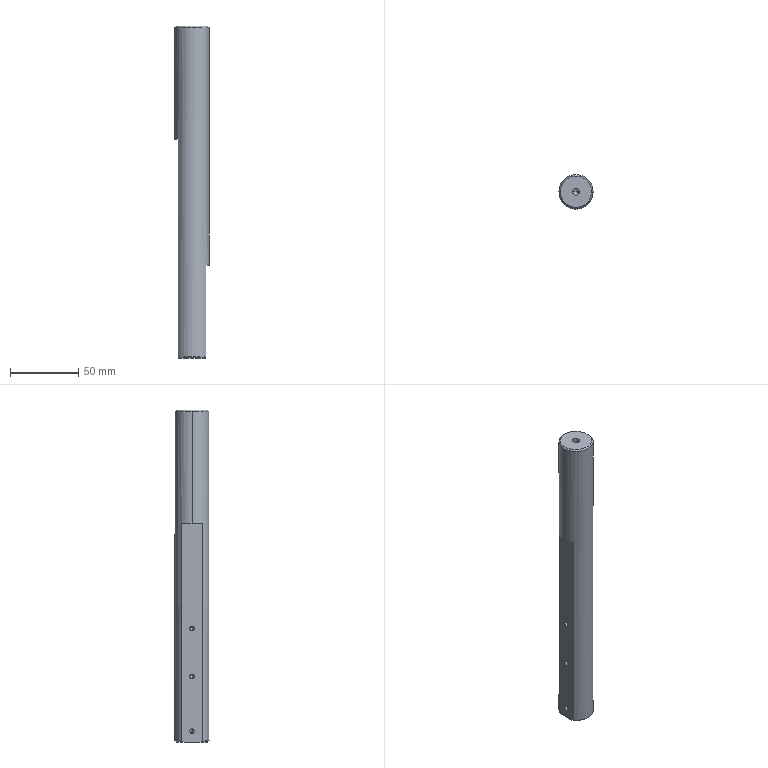Part | SolidWorks | features HoleWzd 3, ICE 3, Chamfer 1, Extrusion 1 | 1 solid | 39 faces | box 25 x 25 x 243 mm | volume 111932 mm3 | cone 16 | cylinder 16 | plane 7 | commonest cylinder face diameters 3.3 x6 5 x6 6 x2 25 x2
STEP:
#1=CARTESIAN_POINT('',(11.5,0.,243.));
#2=VERTEX_POINT('',#1);
#3=CARTESIAN_POINT('',(-11.5,0.,243.));
#4=VERTEX_POINT('',#3);
#5=CARTESIAN_POINT('',(0.,0.,243.));
#6=DIRECTION('',(0.,0.,1.));
#7=DIRECTION('',(1.,0.,0.));
#8=AXIS2_PLACEMENT_3D('',#5,#6,#7);
#9=CIRCLE('',#8,11.5);
#10=EDGE_CURVE('',#2,#4,#9,.T.);
#11=ORIENTED_EDGE('',*,*,#10,.F.);
#12=CARTESIAN_POINT('',(12.5,0.,242.));
#13=VERTEX_POINT('',#12);
#14=CARTESIAN_POINT('',(11.5,0.,243.));
#15=DIRECTION('',(0.7071,0.,-0.7071));
#16=VECTOR('',#15,1000.);
#17=LINE('',#14,#16);
#18=EDGE_CURVE('',#2,#13,#17,.T.);
#19=ORIENTED_EDGE('',*,*,#18,.T.);
#20=CARTESIAN_POINT('',(-12.5,0.,242.));
#21=VERTEX_POINT('',#20);
#22=CARTESIAN_POINT('',(0.,0.,242.));
#23=DIRECTION('',(0.,0.,-1.));
#24=DIRECTION('',(1.,0.,0.));
#25=AXIS2_PLACEMENT_3D('',#22,#23,#24);
#26=CIRCLE('',#25,12.5);
#27=EDGE_CURVE('',#21,#13,#26,.T.);
#28=ORIENTED_EDGE('',*,*,#27,.F.);
#29=CARTESIAN_POINT('',(-11.5,0.,243.));
#30=DIRECTION('',(-0.7071,0.,-0.7071));
#31=VECTOR('',#30,1000.);
#32=LINE('',#29,#31);
#33=EDGE_CURVE('',#4,#21,#32,.T.);
#34=ORIENTED_EDGE('',*,*,#33,.F.);
#35=EDGE_LOOP('',(#11,#19,#28,#34));
#36=FACE_OUTER_BOUND('',#35,.T.);
#37=CARTESIAN_POINT('',(0.,0.,243.));
#38=DIRECTION('',(0.,0.,-1.));
#39=DIRECTION('',(-1.,0.,0.));
#40=AXIS2_PLACEMENT_3D('',#37,#38,#39);
#41=CONICAL_SURFACE('',#40,11.5,0.7854);
#42=ADVANCED_FACE('',(#36),#41,.T.);
#43=CARTESIAN_POINT('',(0.,0.,36.));
#44=VERTEX_POINT('',#43);
#45=CARTESIAN_POINT('',(0.,0.,30.));
#46=VERTEX_POINT('',#45);
#47=CARTESIAN_POINT('',(0.,0.,33.));
#48=DIRECTION('',(1.,0.,0.));
#49=DIRECTION('',(0.,0.,-1.));
#50=AXIS2_PLACEMENT_3D('',#47,#48,#49);
#51=CIRCLE('',#50,3.);
#52=EDGE_CURVE('',#44,#46,#51,.T.);
#53=ORIENTED_EDGE('',*,*,#52,.F.);
#54=CARTESIAN_POINT('',(10.,0.,36.));
#55=VERTEX_POINT('',#54);
#56=CARTESIAN_POINT('',(0.,0.,36.));
#57=DIRECTION('',(1.,0.,0.));
#58=VECTOR('',#57,1000.);
#59=LINE('',#56,#58);
#60=EDGE_CURVE('',#44,#55,#59,.T.);
#61=ORIENTED_EDGE('',*,*,#60,.T.);
#62=CARTESIAN_POINT('',(10.,0.,30.));
#63=VERTEX_POINT('',#62);
#64=CARTESIAN_POINT('',(10.,0.,33.));
#65=DIRECTION('',(1.,0.,0.));
#66=DIRECTION('',(0.,0.,-1.));
#67=AXIS2_PLACEMENT_3D('',#64,#65,#66);
#68=CIRCLE('',#67,3.);
#69=EDGE_CURVE('',#55,#63,#68,.T.);
#70=ORIENTED_EDGE('',*,*,#69,.T.);
#71=CARTESIAN_POINT('',(0.,0.,30.));
#72=DIRECTION('',(1.,0.,0.));
#73=VECTOR('',#72,1000.);
#74=LINE('',#71,#73);
#75=EDGE_CURVE('',#46,#63,#74,.T.);
#76=ORIENTED_EDGE('',*,*,#75,.F.);
#77=EDGE_LOOP('',(#53,#61,#70,#76));
#78=FACE_OUTER_BOUND('',#77,.T.);
#79=CARTESIAN_POINT('',(0.,0.,33.));
#80=DIRECTION('',(1.,0.,0.));
#81=DIRECTION('',(0.,0.,-1.));
#82=AXIS2_PLACEMENT_3D('',#79,#80,#81);
#83=CYLINDRICAL_SURFACE('',#82,3.);
#84=ADVANCED_FACE('',(#78),#83,.F.);
#85=CARTESIAN_POINT('',(0.1,0.,6.35));
#86=VERTEX_POINT('',#85);
#87=CARTESIAN_POINT('',(0.1,0.,9.65));
#88=VERTEX_POINT('',#87);
#89=CARTESIAN_POINT('',(0.1,0.,8.));
#90=DIRECTION('',(-1.,0.,0.));
#91=DIRECTION('',(0.,0.,1.));
#92=AXIS2_PLACEMENT_3D('',#89,#90,#91);
#93=CIRCLE('',#92,1.65);
#94=EDGE_CURVE('',#86,#88,#93,.T.);
#95=ORIENTED_EDGE('',*,*,#94,.F.);
#96=CARTESIAN_POINT('',(-10.,0.,6.35));
#97=VERTEX_POINT('',#96);
#98=CARTESIAN_POINT('',(-10.,0.,6.35));
#99=DIRECTION('',(-1.,0.,0.));
#100=VECTOR('',#99,1000.);
#101=LINE('',#98,#100);
#102=EDGE_CURVE('',#86,#97,#101,.T.);
#103=ORIENTED_EDGE('',*,*,#102,.T.);
#104=CARTESIAN_POINT('',(-10.,0.,9.65));
#105=VERTEX_POINT('',#104);
#106=CARTESIAN_POINT('',(-10.,0.,8.));
#107=DIRECTION('',(-1.,0.,0.));
#108=DIRECTION('',(0.,0.,1.));
#109=AXIS2_PLACEMENT_3D('',#106,#107,#108);
#110=CIRCLE('',#109,1.65);
#111=EDGE_CURVE('',#97,#105,#110,.T.);
#112=ORIENTED_EDGE('',*,*,#111,.T.);
#113=CARTESIAN_POINT('',(-10.,0.,9.65));
#114=DIRECTION('',(-1.,0.,0.));
#115=VECTOR('',#114,1000.);
#116=LINE('',#113,#115);
#117=EDGE_CURVE('',#88,#105,#116,.T.);
#118=ORIENTED_EDGE('',*,*,#117,.F.);
#119=EDGE_LOOP('',(#95,#103,#112,#118));
#120=FACE_OUTER_BOUND('',#119,.T.);
#121=CARTESIAN_POINT('',(-10.,0.,8.));
#122=DIRECTION('',(-1.,0.,0.));
#123=DIRECTION('',(0.,0.,1.));
#124=AXIS2_PLACEMENT_3D('',#121,#122,#123);
#125=CYLINDRICAL_SURFACE('',#124,1.65);
#126=ADVANCED_FACE('',(#120),#125,.F.);
#127=CARTESIAN_POINT('',(1.091,0.,8.));
#128=VERTEX_POINT('',#127);
#129=CARTESIAN_POINT('',(0.1,0.,9.65));
#130=DIRECTION('',(-0.515,0.,0.8572));
#131=VECTOR('',#130,1000.);
#132=LINE('',#129,#131);
#133=EDGE_CURVE('',#128,#88,#132,.T.);
#134=ORIENTED_EDGE('',*,*,#133,.F.);
#135=CARTESIAN_POINT('',(0.1,0.,6.35));
#136=DIRECTION('',(-0.515,0.,-0.8572));
#137=VECTOR('',#136,1000.);
#138=LINE('',#135,#137);
#139=EDGE_CURVE('',#128,#86,#138,.T.);
#140=ORIENTED_EDGE('',*,*,#139,.T.);
#141=ORIENTED_EDGE('',*,*,#94,.T.);
#142=EDGE_LOOP('',(#134,#140,#141));
#143=FACE_OUTER_BOUND('',#142,.T.);
#144=CARTESIAN_POINT('',(0.1,0.,8.));
#145=DIRECTION('',(-1.,0.,0.));
#146=DIRECTION('',(0.,0.,1.));
#147=AXIS2_PLACEMENT_3D('',#144,#145,#146);
#148=CONICAL_SURFACE('',#147,1.65,1.03);
#149=ADVANCED_FACE('',(#143),#148,.F.);
#150=CARTESIAN_POINT('',(0.1,0.,81.35));
#151=VERTEX_POINT('',#150);
#152=CARTESIAN_POINT('',(0.1,0.,84.65));
#153=VERTEX_POINT('',#152);
#154=CARTESIAN_POINT('',(0.1,0.,83.));
#155=DIRECTION('',(-1.,0.,0.));
#156=DIRECTION('',(0.,0.,1.));
#157=AXIS2_PLACEMENT_3D('',#154,#155,#156);
#158=CIRCLE('',#157,1.65);
#159=EDGE_CURVE('',#151,#153,#158,.T.);
#160=ORIENTED_EDGE('',*,*,#159,.F.);
#161=CARTESIAN_POINT('',(-10.,0.,81.35));
#162=VERTEX_POINT('',#161);
#163=CARTESIAN_POINT('',(-10.,0.,81.35));
#164=DIRECTION('',(-1.,0.,0.));
#165=VECTOR('',#164,1000.);
#166=LINE('',#163,#165);
#167=EDGE_CURVE('',#151,#162,#166,.T.);
#168=ORIENTED_EDGE('',*,*,#167,.T.);
#169=CARTESIAN_POINT('',(-10.,0.,84.65));
#170=VERTEX_POINT('',#169);
#171=CARTESIAN_POINT('',(-10.,0.,83.));
#172=DIRECTION('',(-1.,0.,0.));
#173=DIRECTION('',(0.,0.,1.));
#174=AXIS2_PLACEMENT_3D('',#171,#172,#173);
#175=CIRCLE('',#174,1.65);
#176=EDGE_CURVE('',#162,#170,#175,.T.);
#177=ORIENTED_EDGE('',*,*,#176,.T.);
#178=CARTESIAN_POINT('',(-10.,0.,84.65));
#179=DIRECTION('',(-1.,0.,0.));
#180=VECTOR('',#179,1000.);
#181=LINE('',#178,#180);
#182=EDGE_CURVE('',#153,#170,#181,.T.);
#183=ORIENTED_EDGE('',*,*,#182,.F.);
#184=EDGE_LOOP('',(#160,#168,#177,#183));
#185=FACE_OUTER_BOUND('',#184,.T.);
#186=CARTESIAN_POINT('',(-10.,0.,83.));
#187=DIRECTION('',(-1.,0.,0.));
#188=DIRECTION('',(0.,0.,1.));
#189=AXIS2_PLACEMENT_3D('',#186,#187,#188);
#190=CYLINDRICAL_SURFACE('',#189,1.65);
#191=ADVANCED_FACE('',(#185),#190,.F.);
#192=CARTESIAN_POINT('',(1.091,0.,83.));
#193=VERTEX_POINT('',#192);
#194=CARTESIAN_POINT('',(0.1,0.,84.65));
#195=DIRECTION('',(-0.515,0.,0.8572));
#196=VECTOR('',#195,1000.);
#197=LINE('',#194,#196);
#198=EDGE_CURVE('',#193,#153,#197,.T.);
#199=ORIENTED_EDGE('',*,*,#198,.F.);
#200=CARTESIAN_POINT('',(0.1,0.,81.35));
#201=DIRECTION('',(-0.515,0.,-0.8572));
#202=VECTOR('',#201,1000.);
#203=LINE('',#200,#202);
#204=EDGE_CURVE('',#193,#151,#203,.T.);
#205=ORIENTED_EDGE('',*,*,#204,.T.);
#206=ORIENTED_EDGE('',*,*,#159,.T.);
#207=EDGE_LOOP('',(#199,#205,#206));
#208=FACE_OUTER_BOUND('',#207,.T.);
#209=CARTESIAN_POINT('',(0.1,0.,83.));
#210=DIRECTION('',(-1.,0.,0.));
#211=DIRECTION('',(0.,0.,1.));
#212=AXIS2_PLACEMENT_3D('',#209,#210,#211);
#213=CONICAL_SURFACE('',#212,1.65,1.03);
#214=ADVANCED_FACE('',(#208),#213,.F.);
#215=CARTESIAN_POINT('',(0.1,0.,46.35));
#216=VERTEX_POINT('',#215);
#217=CARTESIAN_POINT('',(0.1,0.,49.65));
#218=VERTEX_POINT('',#217);
#219=CARTESIAN_POINT('',(0.1,0.,48.));
#220=DIRECTION('',(-1.,0.,0.));
#221=DIRECTION('',(0.,0.,1.));
#222=AXIS2_PLACEMENT_3D('',#219,#220,#221);
#223=CIRCLE('',#222,1.65);
#224=EDGE_CURVE('',#216,#218,#223,.T.);
#225=ORIENTED_EDGE('',*,*,#224,.F.);
#226=CARTESIAN_POINT('',(-10.,0.,46.35));
#227=VERTEX_POINT('',#226);
#228=CARTESIAN_POINT('',(-10.,0.,46.35));
#229=DIRECTION('',(-1.,0.,0.));
#230=VECTOR('',#229,1000.);
#231=LINE('',#228,#230);
#232=EDGE_CURVE('',#216,#227,#231,.T.);
#233=ORIENTED_EDGE('',*,*,#232,.T.);
#234=CARTESIAN_POINT('',(-10.,0.,49.65));
#235=VERTEX_POINT('',#234);
#236=CARTESIAN_POINT('',(-10.,0.,48.));
#237=DIRECTION('',(-1.,0.,0.));
#238=DIRECTION('',(0.,0.,1.));
#239=AXIS2_PLACEMENT_3D('',#236,#237,#238);
#240=CIRCLE('',#239,1.65);
#241=EDGE_CURVE('',#227,#235,#240,.T.);
#242=ORIENTED_EDGE('',*,*,#241,.T.);
#243=CARTESIAN_POINT('',(-10.,0.,49.65));
#244=DIRECTION('',(-1.,0.,0.));
#245=VECTOR('',#244,1000.);
#246=LINE('',#243,#245);
#247=EDGE_CURVE('',#218,#235,#246,.T.);
#248=ORIENTED_EDGE('',*,*,#247,.F.);
#249=EDGE_LOOP('',(#225,#233,#242,#248));
#250=FACE_OUTER_BOUND('',#249,.T.);
#251=CARTESIAN_POINT('',(-10.,0.,48.));
#252=DIRECTION('',(-1.,0.,0.));
#253=DIRECTION('',(0.,0.,1.));
#254=AXIS2_PLACEMENT_3D('',#251,#252,#253);
#255=CYLINDRICAL_SURFACE('',#254,1.65);
#256=ADVANCED_FACE('',(#250),#255,.F.);
#257=CARTESIAN_POINT('',(1.091,0.,48.));
#258=VERTEX_POINT('',#257);
#259=CARTESIAN_POINT('',(0.1,0.,49.65));
#260=DIRECTION('',(-0.515,0.,0.8572));
#261=VECTOR('',#260,1000.);
#262=LINE('',#259,#261);
#263=EDGE_CURVE('',#258,#218,#262,.T.);
#264=ORIENTED_EDGE('',*,*,#263,.F.);
#265=CARTESIAN_POINT('',(0.1,0.,46.35));
#266=DIRECTION('',(-0.515,0.,-0.8572));
#267=VECTOR('',#266,1000.);
#268=LINE('',#265,#267);
#269=EDGE_CURVE('',#258,#216,#268,.T.);
#270=ORIENTED_EDGE('',*,*,#269,.T.);
#271=ORIENTED_EDGE('',*,*,#224,.T.);
#272=EDGE_LOOP('',(#264,#270,#271));
#273=FACE_OUTER_BOUND('',#272,.T.);
#274=CARTESIAN_POINT('',(0.1,0.,48.));
#275=DIRECTION('',(-1.,0.,0.));
#276=DIRECTION('',(0.,0.,1.));
#277=AXIS2_PLACEMENT_3D('',#274,#275,#276);
#278=CONICAL_SURFACE('',#277,1.65,1.03);
#279=ADVANCED_FACE('',(#273),#278,.F.);
#280=CARTESIAN_POINT('',(-5.,0.,15.5));
#281=VERTEX_POINT('',#280);
#282=CARTESIAN_POINT('',(-5.,0.,10.5));
#283=VERTEX_POINT('',#282);
#284=CARTESIAN_POINT('',(-5.,0.,13.));
#285=DIRECTION('',(1.,0.,0.));
#286=DIRECTION('',(0.,0.,-1.));
#287=AXIS2_PLACEMENT_3D('',#284,#285,#286);
#288=CIRCLE('',#287,2.5);
#289=EDGE_CURVE('',#281,#283,#288,.T.);
#290=ORIENTED_EDGE('',*,*,#289,.F.);
#291=CARTESIAN_POINT('',(10.,0.,15.5));
#292=VERTEX_POINT('',#291);
#293=CARTESIAN_POINT('',(10.,0.,15.5));
#294=DIRECTION('',(1.,0.,0.));
#295=VECTOR('',#294,1000.);
#296=LINE('',#293,#295);
#297=EDGE_CURVE('',#281,#292,#296,.T.);
#298=ORIENTED_EDGE('',*,*,#297,.T.);
#299=CARTESIAN_POINT('',(10.,0.,10.5));
#300=VERTEX_POINT('',#299);
#301=CARTESIAN_POINT('',(10.,0.,13.));
#302=DIRECTION('',(1.,0.,0.));
#303=DIRECTION('',(0.,0.,-1.));
#304=AXIS2_PLACEMENT_3D('',#301,#302,#303);
#305=CIRCLE('',#304,2.5);
#306=EDGE_CURVE('',#292,#300,#305,.T.);
#307=ORIENTED_EDGE('',*,*,#306,.T.);
#308=CARTESIAN_POINT('',(10.,0.,10.5));
#309=DIRECTION('',(1.,0.,0.));
#310=VECTOR('',#309,1000.);
#311=LINE('',#308,#310);
#312=EDGE_CURVE('',#283,#300,#311,.T.);
#313=ORIENTED_EDGE('',*,*,#312,.F.);
#314=EDGE_LOOP('',(#290,#298,#307,#313));
#315=FACE_OUTER_BOUND('',#314,.T.);
#316=CARTESIAN_POINT('',(10.,0.,13.));
#317=DIRECTION('',(1.,0.,0.));
#318=DIRECTION('',(0.,0.,-1.));
#319=AXIS2_PLACEMENT_3D('',#316,#317,#318);
#320=CYLINDRICAL_SURFACE('',#319,2.5);
#321=ADVANCED_FACE('',(#315),#320,.F.);
#322=CARTESIAN_POINT('',(-6.502,0.,13.));
#323=VERTEX_POINT('',#322);
#324=CARTESIAN_POINT('',(-5.,0.,10.5));
#325=DIRECTION('',(0.515,0.,-0.8572));
#326=VECTOR('',#325,1000.);
#327=LINE('',#324,#326);
#328=EDGE_CURVE('',#323,#283,#327,.T.);
#329=ORIENTED_EDGE('',*,*,#328,.F.);
#330=CARTESIAN_POINT('',(-5.,0.,15.5));
#331=DIRECTION('',(0.515,0.,0.8572));
#332=VECTOR('',#331,1000.);
#333=LINE('',#330,#332);
#334=EDGE_CURVE('',#323,#281,#333,.T.);
#335=ORIENTED_EDGE('',*,*,#334,.T.);
#336=ORIENTED_EDGE('',*,*,#289,.T.);
#337=EDGE_LOOP('',(#329,#335,#336));
#338=FACE_OUTER_BOUND('',#337,.T.);
#339=CARTESIAN_POINT('',(-5.,0.,13.));
#340=DIRECTION('',(1.,0.,0.));
#341=DIRECTION('',(0.,0.,-1.));
#342=AXIS2_PLACEMENT_3D('',#339,#340,#341);
#343=CONICAL_SURFACE('',#342,2.5,1.03);
#344=ADVANCED_FACE('',(#338),#343,.F.);
#345=CARTESIAN_POINT('',(-5.,0.,55.5));
#346=VERTEX_POINT('',#345);
#347=CARTESIAN_POINT('',(-5.,0.,50.5));
#348=VERTEX_POINT('',#347);
#349=CARTESIAN_POINT('',(-5.,0.,53.));
#350=DIRECTION('',(1.,0.,0.));
#351=DIRECTION('',(0.,0.,-1.));
#352=AXIS2_PLACEMENT_3D('',#349,#350,#351);
#353=CIRCLE('',#352,2.5);
#354=EDGE_CURVE('',#346,#348,#353,.T.);
#355=ORIENTED_EDGE('',*,*,#354,.F.);
#356=CARTESIAN_POINT('',(10.,0.,55.5));
#357=VERTEX_POINT('',#356);
#358=CARTESIAN_POINT('',(10.,0.,55.5));
#359=DIRECTION('',(1.,0.,0.));
#360=VECTOR('',#359,1000.);
#361=LINE('',#358,#360);
#362=EDGE_CURVE('',#346,#357,#361,.T.);
#363=ORIENTED_EDGE('',*,*,#362,.T.);
#364=CARTESIAN_POINT('',(10.,0.,50.5));
#365=VERTEX_POINT('',#364);
#366=CARTESIAN_POINT('',(10.,0.,53.));
#367=DIRECTION('',(1.,0.,0.));
#368=DIRECTION('',(0.,0.,-1.));
#369=AXIS2_PLACEMENT_3D('',#366,#367,#368);
#370=CIRCLE('',#369,2.5);
#371=EDGE_CURVE('',#357,#365,#370,.T.);
#372=ORIENTED_EDGE('',*,*,#371,.T.);
#373=CARTESIAN_POINT('',(10.,0.,50.5));
#374=DIRECTION('',(1.,0.,0.));
#375=VECTOR('',#374,1000.);
#376=LINE('',#373,#375);
#377=EDGE_CURVE('',#348,#365,#376,.T.);
#378=ORIENTED_EDGE('',*,*,#377,.F.);
#379=EDGE_LOOP('',(#355,#363,#372,#378));
#380=FACE_OUTER_BOUND('',#379,.T.);
#381=CARTESIAN_POINT('',(10.,0.,53.));
#382=DIRECTION('',(1.,0.,0.));
#383=DIRECTION('',(0.,0.,-1.));
#384=AXIS2_PLACEMENT_3D('',#381,#382,#383);
#385=CYLINDRICAL_SURFACE('',#384,2.5);
#386=ADVANCED_FACE('',(#380),#385,.F.);
#387=CARTESIAN_POINT('',(-6.502,0.,53.));
#388=VERTEX_POINT('',#387);
#389=CARTESIAN_POINT('',(-5.,0.,50.5));
#390=DIRECTION('',(0.515,0.,-0.8572));
#391=VECTOR('',#390,1000.);
#392=LINE('',#389,#391);
#393=EDGE_CURVE('',#388,#348,#392,.T.);
#394=ORIENTED_EDGE('',*,*,#393,.F.);
#395=CARTESIAN_POINT('',(-5.,0.,55.5));
#396=DIRECTION('',(0.515,0.,0.8572));
#397=VECTOR('',#396,1000.);
#398=LINE('',#395,#397);
#399=EDGE_CURVE('',#388,#346,#398,.T.);
#400=ORIENTED_EDGE('',*,*,#399,.T.);
#401=ORIENTED_EDGE('',*,*,#354,.T.);
#402=EDGE_LOOP('',(#394,#400,#401));
#403=FACE_OUTER_BOUND('',#402,.T.);
#404=CARTESIAN_POINT('',(-5.,0.,53.));
#405=DIRECTION('',(1.,0.,0.));
#406=DIRECTION('',(0.,0.,-1.));
#407=AXIS2_PLACEMENT_3D('',#404,#405,#406);
#408=CONICAL_SURFACE('',#407,2.5,1.03);
#409=ADVANCED_FACE('',(#403),#408,.F.);
#410=CARTESIAN_POINT('',(-2.5,0.,228.));
#411=VERTEX_POINT('',#410);
#412=CARTESIAN_POINT('',(2.5,0.,228.));
#413=VERTEX_POINT('',#412);
#414=CARTESIAN_POINT('',(0.,0.,228.));
#415=DIRECTION('',(0.,0.,1.));
#416=DIRECTION('',(1.,0.,0.));
#417=AXIS2_PLACEMENT_3D('',#414,#415,#416);
#418=CIRCLE('',#417,2.5);
#419=EDGE_CURVE('',#411,#413,#418,.T.);
#420=ORIENTED_EDGE('',*,*,#419,.F.);
#421=CARTESIAN_POINT('',(-2.5,0.,243.));
#422=VERTEX_POINT('',#421);
#423=CARTESIAN_POINT('',(-2.5,0.,243.));
#424=DIRECTION('',(0.,0.,1.));
#425=VECTOR('',#424,1000.);
#426=LINE('',#423,#425);
#427=EDGE_CURVE('',#411,#422,#426,.T.);
#428=ORIENTED_EDGE('',*,*,#427,.T.);
#429=CARTESIAN_POINT('',(2.5,0.,243.));
#430=VERTEX_POINT('',#429);
#431=CARTESIAN_POINT('',(0.,0.,243.));
#432=DIRECTION('',(0.,0.,1.));
#433=DIRECTION('',(1.,0.,0.));
#434=AXIS2_PLACEMENT_3D('',#431,#432,#433);
#435=CIRCLE('',#434,2.5);
#436=EDGE_CURVE('',#422,#430,#435,.T.);
#437=ORIENTED_EDGE('',*,*,#436,.T.);
#438=CARTESIAN_POINT('',(2.5,0.,243.));
#439=DIRECTION('',(0.,0.,1.));
#440=VECTOR('',#439,1000.);
#441=LINE('',#438,#440);
#442=EDGE_CURVE('',#413,#430,#441,.T.);
#443=ORIENTED_EDGE('',*,*,#442,.F.);
#444=EDGE_LOOP('',(#420,#428,#437,#443));
#445=FACE_OUTER_BOUND('',#444,.T.);
#446=CARTESIAN_POINT('',(0.,0.,243.));
#447=DIRECTION('',(0.,0.,1.));
#448=DIRECTION('',(1.,0.,0.));
#449=AXIS2_PLACEMENT_3D('',#446,#447,#448);
#450=CYLINDRICAL_SURFACE('',#449,2.5);
#451=ADVANCED_FACE('',(#445),#450,.F.);
#452=CARTESIAN_POINT('',(0.,0.,226.498));
#453=VERTEX_POINT('',#452);
#454=CARTESIAN_POINT('',(2.5,0.,228.));
#455=DIRECTION('',(0.8572,0.,0.515));
#456=VECTOR('',#455,1000.);
#457=LINE('',#454,#456);
#458=EDGE_CURVE('',#453,#413,#457,.T.);
#459=ORIENTED_EDGE('',*,*,#458,.F.);
#460=CARTESIAN_POINT('',(-2.5,0.,228.));
#461=DIRECTION('',(-0.8572,0.,0.515));
#462=VECTOR('',#461,1000.);
#463=LINE('',#460,#462);
#464=EDGE_CURVE('',#453,#411,#463,.T.);
#465=ORIENTED_EDGE('',*,*,#464,.T.);
#466=ORIENTED_EDGE('',*,*,#419,.T.);
#467=EDGE_LOOP('',(#459,#465,#466));
#468=FACE_OUTER_BOUND('',#467,.T.);
#469=CARTESIAN_POINT('',(0.,0.,228.));
#470=DIRECTION('',(0.,0.,1.));
#471=DIRECTION('',(1.,0.,0.));
#472=AXIS2_PLACEMENT_3D('',#469,#470,#471);
#473=CONICAL_SURFACE('',#472,2.5,1.03);
#474=ADVANCED_FACE('',(#468),#473,.F.);
#475=ORIENTED_EDGE('',*,*,#27,.T.);
#476=CARTESIAN_POINT('',(12.5,0.,68.));
#477=VERTEX_POINT('',#476);
#478=CARTESIAN_POINT('',(12.5,0.,243.));
#479=DIRECTION('',(0.,0.,-1.));
#480=VECTOR('',#479,1000.);
#481=LINE('',#478,#480);
#482=EDGE_CURVE('',#13,#477,#481,.T.);
#483=ORIENTED_EDGE('',*,*,#482,.T.);
#484=CARTESIAN_POINT('',(10.,7.5,68.));
#485=VERTEX_POINT('',#484);
#486=CARTESIAN_POINT('',(0.,0.,68.));
#487=DIRECTION('',(0.,0.,1.));
#488=DIRECTION('',(1.,0.,0.));
#489=AXIS2_PLACEMENT_3D('',#486,#487,#488);
#490=CIRCLE('',#489,12.5);
#491=EDGE_CURVE('',#477,#485,#490,.T.);
#492=ORIENTED_EDGE('',*,*,#491,.T.);
#493=CARTESIAN_POINT('',(10.,7.5,1.));
#494=VERTEX_POINT('',#493);
#495=CARTESIAN_POINT('',(10.,7.5,68.));
#496=DIRECTION('',(0.,0.,-1.));
#497=VECTOR('',#496,1000.);
#498=LINE('',#495,#497);
#499=EDGE_CURVE('',#485,#494,#498,.T.);
#500=ORIENTED_EDGE('',*,*,#499,.T.);
#501=CARTESIAN_POINT('',(-10.,7.5,1.));
#502=VERTEX_POINT('',#501);
#503=CARTESIAN_POINT('',(0.,0.,1.));
#504=DIRECTION('',(0.,0.,1.));
#505=DIRECTION('',(1.,0.,0.));
#506=AXIS2_PLACEMENT_3D('',#503,#504,#505);
#507=CIRCLE('',#506,12.5);
#508=EDGE_CURVE('',#494,#502,#507,.T.);
#509=ORIENTED_EDGE('',*,*,#508,.T.);
#510=CARTESIAN_POINT('',(-10.,7.5,160.));
#511=VERTEX_POINT('',#510);
#512=CARTESIAN_POINT('',(-10.,7.5,160.));
#513=DIRECTION('',(0.,0.,-1.));
#514=VECTOR('',#513,1000.);
#515=LINE('',#512,#514);
#516=EDGE_CURVE('',#511,#502,#515,.T.);
#517=ORIENTED_EDGE('',*,*,#516,.F.);
#518=CARTESIAN_POINT('',(-12.5,0.,160.));
#519=VERTEX_POINT('',#518);
#520=CARTESIAN_POINT('',(0.,0.,160.));
#521=DIRECTION('',(0.,0.,1.));
#522=DIRECTION('',(1.,0.,0.));
#523=AXIS2_PLACEMENT_3D('',#520,#521,#522);
#524=CIRCLE('',#523,12.5);
#525=EDGE_CURVE('',#511,#519,#524,.T.);
#526=ORIENTED_EDGE('',*,*,#525,.T.);
#527=CARTESIAN_POINT('',(-12.5,0.,243.));
#528=DIRECTION('',(0.,0.,-1.));
#529=VECTOR('',#528,1000.);
#530=LINE('',#527,#529);
#531=EDGE_CURVE('',#21,#519,#530,.T.);
#532=ORIENTED_EDGE('',*,*,#531,.F.);
#533=EDGE_LOOP('',(#475,#483,#492,#500,#509,#517,#526,#532));
#534=FACE_OUTER_BOUND('',#533,.T.);
#535=CARTESIAN_POINT('',(0.,0.,243.));
#536=DIRECTION('',(0.,0.,-1.));
#537=DIRECTION('',(-1.,0.,0.));
#538=AXIS2_PLACEMENT_3D('',#535,#536,#537);
#539=CYLINDRICAL_SURFACE('',#538,12.5);
#540=ADVANCED_FACE('',(#534),#539,.T.);
#541=ORIENTED_EDGE('',*,*,#482,.F.);
#542=CARTESIAN_POINT('',(0.,0.,242.));
#543=DIRECTION('',(0.,0.,-1.));
#544=DIRECTION('',(1.,0.,0.));
#545=AXIS2_PLACEMENT_3D('',#542,#543,#544);
#546=CIRCLE('',#545,12.5);
#547=EDGE_CURVE('',#13,#21,#546,.T.);
#548=ORIENTED_EDGE('',*,*,#547,.T.);
#549=ORIENTED_EDGE('',*,*,#531,.T.);
#550=CARTESIAN_POINT('',(-10.,-7.5,160.));
#551=VERTEX_POINT('',#550);
#552=CARTESIAN_POINT('',(0.,0.,160.));
#553=DIRECTION('',(0.,0.,1.));
#554=DIRECTION('',(1.,0.,0.));
#555=AXIS2_PLACEMENT_3D('',#552,#553,#554);
#556=CIRCLE('',#555,12.5);
#557=EDGE_CURVE('',#519,#551,#556,.T.);
#558=ORIENTED_EDGE('',*,*,#557,.T.);
#559=CARTESIAN_POINT('',(-10.,-7.5,1.));
#560=VERTEX_POINT('',#559);
#561=CARTESIAN_POINT('',(-10.,-7.5,160.));
#562=DIRECTION('',(0.,0.,-1.));
#563=VECTOR('',#562,1000.);
#564=LINE('',#561,#563);
#565=EDGE_CURVE('',#551,#560,#564,.T.);
#566=ORIENTED_EDGE('',*,*,#565,.T.);
#567=CARTESIAN_POINT('',(10.,-7.5,1.));
#568=VERTEX_POINT('',#567);
#569=CARTESIAN_POINT('',(0.,0.,1.));
#570=DIRECTION('',(0.,0.,1.));
#571=DIRECTION('',(1.,0.,0.));
#572=AXIS2_PLACEMENT_3D('',#569,#570,#571);
#573=CIRCLE('',#572,12.5);
#574=EDGE_CURVE('',#560,#568,#573,.T.);
#575=ORIENTED_EDGE('',*,*,#574,.T.);
#576=CARTESIAN_POINT('',(10.,-7.5,68.));
#577=VERTEX_POINT('',#576);
#578=CARTESIAN_POINT('',(10.,-7.5,68.));
#579=DIRECTION('',(0.,0.,-1.));
#580=VECTOR('',#579,1000.);
#581=LINE('',#578,#580);
#582=EDGE_CURVE('',#577,#568,#581,.T.);
#583=ORIENTED_EDGE('',*,*,#582,.F.);
#584=CARTESIAN_POINT('',(0.,0.,68.));
#585=DIRECTION('',(0.,0.,1.));
#586=DIRECTION('',(1.,0.,0.));
#587=AXIS2_PLACEMENT_3D('',#584,#585,#586);
#588=CIRCLE('',#587,12.5);
#589=EDGE_CURVE('',#577,#477,#588,.T.);
#590=ORIENTED_EDGE('',*,*,#589,.T.);
#591=EDGE_LOOP('',(#541,#548,#549,#558,#566,#575,#583,#590));
#592=FACE_OUTER_BOUND('',#591,.T.);
#593=CARTESIAN_POINT('',(0.,0.,243.));
#594=DIRECTION('',(0.,0.,-1.));
#595=DIRECTION('',(-1.,0.,0.));
#596=AXIS2_PLACEMENT_3D('',#593,#594,#595);
#597=CYLINDRICAL_SURFACE('',#596,12.5);
#598=ADVANCED_FACE('',(#592),#597,.T.);
#599=CARTESIAN_POINT('',(10.,5.679,0.));
#600=VERTEX_POINT('',#599);
#601=CARTESIAN_POINT('',(10.,-5.679,0.));
#602=VERTEX_POINT('',#601);
#603=CARTESIAN_POINT('',(10.,7.5,0.));
#604=DIRECTION('',(0.,-1.,0.));
#605=VECTOR('',#604,1000.);
#606=LINE('',#603,#605);
#607=EDGE_CURVE('',#600,#602,#606,.T.);
#608=ORIENTED_EDGE('',*,*,#607,.T.);
#609=CARTESIAN_POINT('',(-10.,-5.679,0.));
#610=VERTEX_POINT('',#609);
#611=CARTESIAN_POINT('',(0.,0.,0.));
#612=DIRECTION('',(0.,0.,-1.));
#613=DIRECTION('',(1.,0.,0.));
#614=AXIS2_PLACEMENT_3D('',#611,#612,#613);
#615=CIRCLE('',#614,11.5);
#616=EDGE_CURVE('',#602,#610,#615,.T.);
#617=ORIENTED_EDGE('',*,*,#616,.T.);
#618=CARTESIAN_POINT('',(-10.,5.679,0.));
#619=VERTEX_POINT('',#618);
#620=CARTESIAN_POINT('',(-10.,-7.5,0.));
#621=DIRECTION('',(0.,-1.,0.));
#622=VECTOR('',#621,1000.);
#623=LINE('',#620,#622);
#624=EDGE_CURVE('',#619,#610,#623,.T.);
#625=ORIENTED_EDGE('',*,*,#624,.F.);
#626=CARTESIAN_POINT('',(0.,0.,0.));
#627=DIRECTION('',(0.,0.,-1.));
#628=DIRECTION('',(1.,0.,0.));
#629=AXIS2_PLACEMENT_3D('',#626,#627,#628);
#630=CIRCLE('',#629,11.5);
#631=EDGE_CURVE('',#619,#600,#630,.T.);
#632=ORIENTED_EDGE('',*,*,#631,.T.);
#633=EDGE_LOOP('',(#608,#617,#625,#632));
#634=FACE_OUTER_BOUND('',#633,.T.);
#635=CARTESIAN_POINT('',(0.,0.,0.));
#636=DIRECTION('',(0.,0.,1.));
#637=DIRECTION('',(1.,0.,0.));
#638=AXIS2_PLACEMENT_3D('',#635,#636,#637);
#639=PLANE('',#638);
#640=ADVANCED_FACE('',(#634),#639,.F.);
#641=CARTESIAN_POINT('',(0.,0.,243.));
#642=DIRECTION('',(0.,0.,1.));
#643=DIRECTION('',(1.,0.,0.));
#644=AXIS2_PLACEMENT_3D('',#641,#642,#643);
#645=CIRCLE('',#644,11.5);
#646=EDGE_CURVE('',#4,#2,#645,.T.);
#647=ORIENTED_EDGE('',*,*,#646,.T.);
#648=ORIENTED_EDGE('',*,*,#10,.T.);
#649=EDGE_LOOP('',(#647,#648));
#650=FACE_OUTER_BOUND('',#649,.T.);
#651=CARTESIAN_POINT('',(0.,0.,243.));
#652=DIRECTION('',(0.,0.,1.));
#653=DIRECTION('',(1.,0.,0.));
#654=AXIS2_PLACEMENT_3D('',#651,#652,#653);
#655=CIRCLE('',#654,2.5);
#656=EDGE_CURVE('',#430,#422,#655,.T.);
#657=ORIENTED_EDGE('',*,*,#656,.F.);
#658=ORIENTED_EDGE('',*,*,#436,.F.);
#659=EDGE_LOOP('',(#657,#658));
#660=FACE_BOUND('',#659,.T.);
#661=CARTESIAN_POINT('',(0.,0.,243.));
#662=DIRECTION('',(0.,0.,1.));
#663=DIRECTION('',(1.,0.,0.));
#664=AXIS2_PLACEMENT_3D('',#661,#662,#663);
#665=PLANE('',#664);
#666=ADVANCED_FACE('',(#650,#660),#665,.T.);
#667=CARTESIAN_POINT('',(10.,7.5,68.));
#668=DIRECTION('',(0.,-1.,0.));
#669=VECTOR('',#668,1000.);
#670=LINE('',#667,#669);
#671=EDGE_CURVE('',#485,#577,#670,.T.);
#672=ORIENTED_EDGE('',*,*,#671,.F.);
#673=ORIENTED_EDGE('',*,*,#491,.F.);
#674=ORIENTED_EDGE('',*,*,#589,.F.);
#675=EDGE_LOOP('',(#672,#673,#674));
#676=FACE_OUTER_BOUND('',#675,.T.);
#677=CARTESIAN_POINT('',(0.,0.,68.));
#678=DIRECTION('',(0.,0.,1.));
#679=DIRECTION('',(1.,0.,0.));
#680=AXIS2_PLACEMENT_3D('',#677,#678,#679);
#681=PLANE('',#680);
#682=ADVANCED_FACE('',(#676),#681,.F.);
#683=CARTESIAN_POINT('',(10.,0.,33.));
#684=DIRECTION('',(1.,0.,0.));
#685=DIRECTION('',(0.,0.,-1.));
#686=AXIS2_PLACEMENT_3D('',#683,#684,#685);
#687=CIRCLE('',#686,3.);
#688=EDGE_CURVE('',#63,#55,#687,.T.);
#689=ORIENTED_EDGE('',*,*,#688,.F.);
#690=ORIENTED_EDGE('',*,*,#69,.F.);
#691=EDGE_LOOP('',(#689,#690));
#692=FACE_BOUND('',#691,.T.);
#693=CARTESIAN_POINT('',(10.,0.,13.));
#694=DIRECTION('',(1.,0.,0.));
#695=DIRECTION('',(0.,0.,-1.));
#696=AXIS2_PLACEMENT_3D('',#693,#694,#695);
#697=CIRCLE('',#696,2.5);
#698=EDGE_CURVE('',#300,#292,#697,.T.);
#699=ORIENTED_EDGE('',*,*,#698,.F.);
#700=ORIENTED_EDGE('',*,*,#306,.F.);
#701=EDGE_LOOP('',(#699,#700));
#702=FACE_BOUND('',#701,.T.);
#703=CARTESIAN_POINT('',(10.,0.,53.));
#704=DIRECTION('',(1.,0.,0.));
#705=DIRECTION('',(0.,0.,-1.));
#706=AXIS2_PLACEMENT_3D('',#703,#704,#705);
#707=CIRCLE('',#706,2.5);
#708=EDGE_CURVE('',#365,#357,#707,.T.);
#709=ORIENTED_EDGE('',*,*,#708,.F.);
#710=ORIENTED_EDGE('',*,*,#371,.F.);
#711=EDGE_LOOP('',(#709,#710));
#712=FACE_BOUND('',#711,.T.);
#713=ORIENTED_EDGE('',*,*,#582,.T.);
#714=CARTESIAN_POINT('',(10.,-7.5,1.));
#715=CARTESIAN_POINT('',(10.,-6.906,0.6434));
#716=CARTESIAN_POINT('',(10.,-6.3,0.3069));
#717=CARTESIAN_POINT('',(10.,-5.679,0.));
#718=B_SPLINE_CURVE_WITH_KNOTS('',3,(#714,#715,#716,#717),.UNSPECIFIED.,.F.,.F.,(4,4),(0.,0.002078),.UNSPECIFIED.);
#719=EDGE_CURVE('',#568,#602,#718,.T.);
#720=ORIENTED_EDGE('',*,*,#719,.T.);
#721=ORIENTED_EDGE('',*,*,#607,.F.);
#722=CARTESIAN_POINT('',(10.,5.679,0.));
#723=CARTESIAN_POINT('',(10.,6.3,0.3069));
#724=CARTESIAN_POINT('',(10.,6.906,0.6434));
#725=CARTESIAN_POINT('',(10.,7.5,1.));
#726=B_SPLINE_CURVE_WITH_KNOTS('',3,(#722,#723,#724,#725),.UNSPECIFIED.,.F.,.F.,(4,4),(0.,0.002078),.UNSPECIFIED.);
#727=EDGE_CURVE('',#600,#494,#726,.T.);
#728=ORIENTED_EDGE('',*,*,#727,.T.);
#729=ORIENTED_EDGE('',*,*,#499,.F.);
#730=ORIENTED_EDGE('',*,*,#671,.T.);
#731=EDGE_LOOP('',(#713,#720,#721,#728,#729,#730));
#732=FACE_OUTER_BOUND('',#731,.T.);
#733=CARTESIAN_POINT('',(10.,7.5,68.));
#734=DIRECTION('',(1.,0.,0.));
#735=DIRECTION('',(0.,0.,-1.));
#736=AXIS2_PLACEMENT_3D('',#733,#734,#735);
#737=PLANE('',#736);
#738=ADVANCED_FACE('',(#692,#702,#712,#732),#737,.T.);
#739=ORIENTED_EDGE('',*,*,#464,.F.);
#740=ORIENTED_EDGE('',*,*,#458,.T.);
#741=CARTESIAN_POINT('',(0.,0.,228.));
#742=DIRECTION('',(0.,0.,1.));
#743=DIRECTION('',(1.,0.,0.));
#744=AXIS2_PLACEMENT_3D('',#741,#742,#743);
#745=CIRCLE('',#744,2.5);
#746=EDGE_CURVE('',#413,#411,#745,.T.);
#747=ORIENTED_EDGE('',*,*,#746,.T.);
#748=EDGE_LOOP('',(#739,#740,#747));
#749=FACE_OUTER_BOUND('',#748,.T.);
#750=CARTESIAN_POINT('',(0.,0.,228.));
#751=DIRECTION('',(0.,0.,1.));
#752=DIRECTION('',(1.,0.,0.));
#753=AXIS2_PLACEMENT_3D('',#750,#751,#752);
#754=CONICAL_SURFACE('',#753,2.5,1.03);
#755=ADVANCED_FACE('',(#749),#754,.F.);
#756=ORIENTED_EDGE('',*,*,#427,.F.);
#757=ORIENTED_EDGE('',*,*,#746,.F.);
#758=ORIENTED_EDGE('',*,*,#442,.T.);
#759=ORIENTED_EDGE('',*,*,#656,.T.);
#760=EDGE_LOOP('',(#756,#757,#758,#759));
#761=FACE_OUTER_BOUND('',#760,.T.);
#762=CARTESIAN_POINT('',(0.,0.,243.));
#763=DIRECTION('',(0.,0.,1.));
#764=DIRECTION('',(1.,0.,0.));
#765=AXIS2_PLACEMENT_3D('',#762,#763,#764);
#766=CYLINDRICAL_SURFACE('',#765,2.5);
#767=ADVANCED_FACE('',(#761),#766,.F.);
#768=ORIENTED_EDGE('',*,*,#399,.F.);
#769=ORIENTED_EDGE('',*,*,#393,.T.);
#770=CARTESIAN_POINT('',(-5.,0.,53.));
#771=DIRECTION('',(1.,0.,0.));
#772=DIRECTION('',(0.,0.,-1.));
#773=AXIS2_PLACEMENT_3D('',#770,#771,#772);
#774=CIRCLE('',#773,2.5);
#775=EDGE_CURVE('',#348,#346,#774,.T.);
#776=ORIENTED_EDGE('',*,*,#775,.T.);
#777=EDGE_LOOP('',(#768,#769,#776));
#778=FACE_OUTER_BOUND('',#777,.T.);
#779=CARTESIAN_POINT('',(-5.,0.,53.));
#780=DIRECTION('',(1.,0.,0.));
#781=DIRECTION('',(0.,0.,-1.));
#782=AXIS2_PLACEMENT_3D('',#779,#780,#781);
#783=CONICAL_SURFACE('',#782,2.5,1.03);
#784=ADVANCED_FACE('',(#778),#783,.F.);
#785=ORIENTED_EDGE('',*,*,#362,.F.);
#786=ORIENTED_EDGE('',*,*,#775,.F.);
#787=ORIENTED_EDGE('',*,*,#377,.T.);
#788=ORIENTED_EDGE('',*,*,#708,.T.);
#789=EDGE_LOOP('',(#785,#786,#787,#788));
#790=FACE_OUTER_BOUND('',#789,.T.);
#791=CARTESIAN_POINT('',(10.,0.,53.));
#792=DIRECTION('',(1.,0.,0.));
#793=DIRECTION('',(0.,0.,-1.));
#794=AXIS2_PLACEMENT_3D('',#791,#792,#793);
#795=CYLINDRICAL_SURFACE('',#794,2.5);
#796=ADVANCED_FACE('',(#790),#795,.F.);
#797=ORIENTED_EDGE('',*,*,#334,.F.);
#798=ORIENTED_EDGE('',*,*,#328,.T.);
#799=CARTESIAN_POINT('',(-5.,0.,13.));
#800=DIRECTION('',(1.,0.,0.));
#801=DIRECTION('',(0.,0.,-1.));
#802=AXIS2_PLACEMENT_3D('',#799,#800,#801);
#803=CIRCLE('',#802,2.5);
#804=EDGE_CURVE('',#283,#281,#803,.T.);
#805=ORIENTED_EDGE('',*,*,#804,.T.);
#806=EDGE_LOOP('',(#797,#798,#805));
#807=FACE_OUTER_BOUND('',#806,.T.);
#808=CARTESIAN_POINT('',(-5.,0.,13.));
#809=DIRECTION('',(1.,0.,0.));
#810=DIRECTION('',(0.,0.,-1.));
#811=AXIS2_PLACEMENT_3D('',#808,#809,#810);
#812=CONICAL_SURFACE('',#811,2.5,1.03);
#813=ADVANCED_FACE('',(#807),#812,.F.);
#814=ORIENTED_EDGE('',*,*,#297,.F.);
#815=ORIENTED_EDGE('',*,*,#804,.F.);
#816=ORIENTED_EDGE('',*,*,#312,.T.);
#817=ORIENTED_EDGE('',*,*,#698,.T.);
#818=EDGE_LOOP('',(#814,#815,#816,#817));
#819=FACE_OUTER_BOUND('',#818,.T.);
#820=CARTESIAN_POINT('',(10.,0.,13.));
#821=DIRECTION('',(1.,0.,0.));
#822=DIRECTION('',(0.,0.,-1.));
#823=AXIS2_PLACEMENT_3D('',#820,#821,#822);
#824=CYLINDRICAL_SURFACE('',#823,2.5);
#825=ADVANCED_FACE('',(#819),#824,.F.);
#826=CARTESIAN_POINT('',(-10.,-7.5,160.));
#827=DIRECTION('',(0.,-1.,0.));
#828=VECTOR('',#827,1000.);
#829=LINE('',#826,#828);
#830=EDGE_CURVE('',#511,#551,#829,.T.);
#831=ORIENTED_EDGE('',*,*,#830,.T.);
#832=ORIENTED_EDGE('',*,*,#557,.F.);
#833=ORIENTED_EDGE('',*,*,#525,.F.);
#834=EDGE_LOOP('',(#831,#832,#833));
#835=FACE_OUTER_BOUND('',#834,.T.);
#836=CARTESIAN_POINT('',(0.,0.,160.));
#837=DIRECTION('',(0.,0.,1.));
#838=DIRECTION('',(1.,0.,0.));
#839=AXIS2_PLACEMENT_3D('',#836,#837,#838);
#840=PLANE('',#839);
#841=ADVANCED_FACE('',(#835),#840,.F.);
#842=CARTESIAN_POINT('',(-10.,0.,8.));
#843=DIRECTION('',(-1.,0.,0.));
#844=DIRECTION('',(0.,0.,1.));
#845=AXIS2_PLACEMENT_3D('',#842,#843,#844);
#846=CIRCLE('',#845,1.65);
#847=EDGE_CURVE('',#105,#97,#846,.T.);
#848=ORIENTED_EDGE('',*,*,#847,.F.);
#849=ORIENTED_EDGE('',*,*,#111,.F.);
#850=EDGE_LOOP('',(#848,#849));
#851=FACE_BOUND('',#850,.T.);
#852=CARTESIAN_POINT('',(-10.,0.,83.));
#853=DIRECTION('',(-1.,0.,0.));
#854=DIRECTION('',(0.,0.,1.));
#855=AXIS2_PLACEMENT_3D('',#852,#853,#854);
#856=CIRCLE('',#855,1.65);
#857=EDGE_CURVE('',#170,#162,#856,.T.);
#858=ORIENTED_EDGE('',*,*,#857,.F.);
#859=ORIENTED_EDGE('',*,*,#176,.F.);
#860=EDGE_LOOP('',(#858,#859));
#861=FACE_BOUND('',#860,.T.);
#862=CARTESIAN_POINT('',(-10.,0.,48.));
#863=DIRECTION('',(-1.,0.,0.));
#864=DIRECTION('',(0.,0.,1.));
#865=AXIS2_PLACEMENT_3D('',#862,#863,#864);
#866=CIRCLE('',#865,1.65);
#867=EDGE_CURVE('',#235,#227,#866,.T.);
#868=ORIENTED_EDGE('',*,*,#867,.F.);
#869=ORIENTED_EDGE('',*,*,#241,.F.);
#870=EDGE_LOOP('',(#868,#869));
#871=FACE_BOUND('',#870,.T.);
#872=ORIENTED_EDGE('',*,*,#624,.T.);
#873=CARTESIAN_POINT('',(-10.,-5.679,0.));
#874=CARTESIAN_POINT('',(-10.,-6.3,0.3069));
#875=CARTESIAN_POINT('',(-10.,-6.906,0.6434));
#876=CARTESIAN_POINT('',(-10.,-7.5,1.));
#877=B_SPLINE_CURVE_WITH_KNOTS('',3,(#873,#874,#875,#876),.UNSPECIFIED.,.F.,.F.,(4,4),(0.,0.002078),.UNSPECIFIED.);
#878=EDGE_CURVE('',#610,#560,#877,.T.);
#879=ORIENTED_EDGE('',*,*,#878,.T.);
#880=ORIENTED_EDGE('',*,*,#565,.F.);
#881=ORIENTED_EDGE('',*,*,#830,.F.);
#882=ORIENTED_EDGE('',*,*,#516,.T.);
#883=CARTESIAN_POINT('',(-10.,7.5,1.));
#884=CARTESIAN_POINT('',(-10.,6.906,0.6434));
#885=CARTESIAN_POINT('',(-10.,6.3,0.3069));
#886=CARTESIAN_POINT('',(-10.,5.679,0.));
#887=B_SPLINE_CURVE_WITH_KNOTS('',3,(#883,#884,#885,#886),.UNSPECIFIED.,.F.,.F.,(4,4),(0.,0.002078),.UNSPECIFIED.);
#888=EDGE_CURVE('',#502,#619,#887,.T.);
#889=ORIENTED_EDGE('',*,*,#888,.T.);
#890=EDGE_LOOP('',(#872,#879,#880,#881,#882,#889));
#891=FACE_OUTER_BOUND('',#890,.T.);
#892=CARTESIAN_POINT('',(-10.,-7.5,160.));
#893=DIRECTION('',(1.,0.,0.));
#894=DIRECTION('',(0.,0.,-1.));
#895=AXIS2_PLACEMENT_3D('',#892,#893,#894);
#896=PLANE('',#895);
#897=ADVANCED_FACE('',(#851,#861,#871,#891),#896,.F.);
#898=ORIENTED_EDGE('',*,*,#269,.F.);
#899=ORIENTED_EDGE('',*,*,#263,.T.);
#900=CARTESIAN_POINT('',(0.1,0.,48.));
#901=DIRECTION('',(-1.,0.,0.));
#902=DIRECTION('',(0.,0.,1.));
#903=AXIS2_PLACEMENT_3D('',#900,#901,#902);
#904=CIRCLE('',#903,1.65);
#905=EDGE_CURVE('',#218,#216,#904,.T.);
#906=ORIENTED_EDGE('',*,*,#905,.T.);
#907=EDGE_LOOP('',(#898,#899,#906));
#908=FACE_OUTER_BOUND('',#907,.T.);
#909=CARTESIAN_POINT('',(0.1,0.,48.));
#910=DIRECTION('',(-1.,0.,0.));
#911=DIRECTION('',(0.,0.,1.));
#912=AXIS2_PLACEMENT_3D('',#909,#910,#911);
#913=CONICAL_SURFACE('',#912,1.65,1.03);
#914=ADVANCED_FACE('',(#908),#913,.F.);
#915=ORIENTED_EDGE('',*,*,#232,.F.);
#916=ORIENTED_EDGE('',*,*,#905,.F.);
#917=ORIENTED_EDGE('',*,*,#247,.T.);
#918=ORIENTED_EDGE('',*,*,#867,.T.);
#919=EDGE_LOOP('',(#915,#916,#917,#918));
#920=FACE_OUTER_BOUND('',#919,.T.);
#921=CARTESIAN_POINT('',(-10.,0.,48.));
#922=DIRECTION('',(-1.,0.,0.));
#923=DIRECTION('',(0.,0.,1.));
#924=AXIS2_PLACEMENT_3D('',#921,#922,#923);
#925=CYLINDRICAL_SURFACE('',#924,1.65);
#926=ADVANCED_FACE('',(#920),#925,.F.);
#927=ORIENTED_EDGE('',*,*,#204,.F.);
#928=ORIENTED_EDGE('',*,*,#198,.T.);
#929=CARTESIAN_POINT('',(0.1,0.,83.));
#930=DIRECTION('',(-1.,0.,0.));
#931=DIRECTION('',(0.,0.,1.));
#932=AXIS2_PLACEMENT_3D('',#929,#930,#931);
#933=CIRCLE('',#932,1.65);
#934=EDGE_CURVE('',#153,#151,#933,.T.);
#935=ORIENTED_EDGE('',*,*,#934,.T.);
#936=EDGE_LOOP('',(#927,#928,#935));
#937=FACE_OUTER_BOUND('',#936,.T.);
#938=CARTESIAN_POINT('',(0.1,0.,83.));
#939=DIRECTION('',(-1.,0.,0.));
#940=DIRECTION('',(0.,0.,1.));
#941=AXIS2_PLACEMENT_3D('',#938,#939,#940);
#942=CONICAL_SURFACE('',#941,1.65,1.03);
#943=ADVANCED_FACE('',(#937),#942,.F.);
#944=ORIENTED_EDGE('',*,*,#167,.F.);
#945=ORIENTED_EDGE('',*,*,#934,.F.);
#946=ORIENTED_EDGE('',*,*,#182,.T.);
#947=ORIENTED_EDGE('',*,*,#857,.T.);
#948=EDGE_LOOP('',(#944,#945,#946,#947));
#949=FACE_OUTER_BOUND('',#948,.T.);
#950=CARTESIAN_POINT('',(-10.,0.,83.));
#951=DIRECTION('',(-1.,0.,0.));
#952=DIRECTION('',(0.,0.,1.));
#953=AXIS2_PLACEMENT_3D('',#950,#951,#952);
#954=CYLINDRICAL_SURFACE('',#953,1.65);
#955=ADVANCED_FACE('',(#949),#954,.F.);
#956=ORIENTED_EDGE('',*,*,#139,.F.);
#957=ORIENTED_EDGE('',*,*,#133,.T.);
#958=CARTESIAN_POINT('',(0.1,0.,8.));
#959=DIRECTION('',(-1.,0.,0.));
#960=DIRECTION('',(0.,0.,1.));
#961=AXIS2_PLACEMENT_3D('',#958,#959,#960);
#962=CIRCLE('',#961,1.65);
#963=EDGE_CURVE('',#88,#86,#962,.T.);
#964=ORIENTED_EDGE('',*,*,#963,.T.);
#965=EDGE_LOOP('',(#956,#957,#964));
#966=FACE_OUTER_BOUND('',#965,.T.);
#967=CARTESIAN_POINT('',(0.1,0.,8.));
#968=DIRECTION('',(-1.,0.,0.));
#969=DIRECTION('',(0.,0.,1.));
#970=AXIS2_PLACEMENT_3D('',#967,#968,#969);
#971=CONICAL_SURFACE('',#970,1.65,1.03);
#972=ADVANCED_FACE('',(#966),#971,.F.);
#973=ORIENTED_EDGE('',*,*,#102,.F.);
#974=ORIENTED_EDGE('',*,*,#963,.F.);
#975=ORIENTED_EDGE('',*,*,#117,.T.);
#976=ORIENTED_EDGE('',*,*,#847,.T.);
#977=EDGE_LOOP('',(#973,#974,#975,#976));
#978=FACE_OUTER_BOUND('',#977,.T.);
#979=CARTESIAN_POINT('',(-10.,0.,8.));
#980=DIRECTION('',(-1.,0.,0.));
#981=DIRECTION('',(0.,0.,1.));
#982=AXIS2_PLACEMENT_3D('',#979,#980,#981);
#983=CYLINDRICAL_SURFACE('',#982,1.65);
#984=ADVANCED_FACE('',(#978),#983,.F.);
#985=ORIENTED_EDGE('',*,*,#60,.F.);
#986=CARTESIAN_POINT('',(0.,0.,33.));
#987=DIRECTION('',(1.,0.,0.));
#988=DIRECTION('',(0.,0.,-1.));
#989=AXIS2_PLACEMENT_3D('',#986,#987,#988);
#990=CIRCLE('',#989,3.);
#991=EDGE_CURVE('',#46,#44,#990,.T.);
#992=ORIENTED_EDGE('',*,*,#991,.F.);
#993=ORIENTED_EDGE('',*,*,#75,.T.);
#994=ORIENTED_EDGE('',*,*,#688,.T.);
#995=EDGE_LOOP('',(#985,#992,#993,#994));
#996=FACE_OUTER_BOUND('',#995,.T.);
#997=CARTESIAN_POINT('',(0.,0.,33.));
#998=DIRECTION('',(1.,0.,0.));
#999=DIRECTION('',(0.,0.,-1.));
#1000=AXIS2_PLACEMENT_3D('',#997,#998,#999);
#1001=CYLINDRICAL_SURFACE('',#1000,3.);
#1002=ADVANCED_FACE('',(#996),#1001,.F.);
#1003=ORIENTED_EDGE('',*,*,#991,.T.);
#1004=ORIENTED_EDGE('',*,*,#52,.T.);
#1005=EDGE_LOOP('',(#1003,#1004));
#1006=FACE_OUTER_BOUND('',#1005,.T.);
#1007=CARTESIAN_POINT('',(0.,0.,33.));
#1008=DIRECTION('',(1.,0.,0.));
#1009=DIRECTION('',(0.,0.,-1.));
#1010=AXIS2_PLACEMENT_3D('',#1007,#1008,#1009);
#1011=PLANE('',#1010);
#1012=ADVANCED_FACE('',(#1006),#1011,.T.);
#1013=ORIENTED_EDGE('',*,*,#878,.F.);
#1014=ORIENTED_EDGE('',*,*,#616,.F.);
#1015=ORIENTED_EDGE('',*,*,#719,.F.);
#1016=ORIENTED_EDGE('',*,*,#574,.F.);
#1017=EDGE_LOOP('',(#1013,#1014,#1015,#1016));
#1018=FACE_OUTER_BOUND('',#1017,.T.);
#1019=CARTESIAN_POINT('',(0.,0.,1.));
#1020=DIRECTION('',(0.,0.,1.));
#1021=DIRECTION('',(1.,0.,0.));
#1022=AXIS2_PLACEMENT_3D('',#1019,#1020,#1021);
#1023=CONICAL_SURFACE('',#1022,12.5,0.7854);
#1024=ADVANCED_FACE('',(#1018),#1023,.T.);
#1025=ORIENTED_EDGE('',*,*,#727,.F.);
#1026=ORIENTED_EDGE('',*,*,#631,.F.);
#1027=ORIENTED_EDGE('',*,*,#888,.F.);
#1028=ORIENTED_EDGE('',*,*,#508,.F.);
#1029=EDGE_LOOP('',(#1025,#1026,#1027,#1028));
#1030=FACE_OUTER_BOUND('',#1029,.T.);
#1031=CARTESIAN_POINT('',(0.,0.,1.));
#1032=DIRECTION('',(0.,0.,1.));
#1033=DIRECTION('',(1.,0.,0.));
#1034=AXIS2_PLACEMENT_3D('',#1031,#1032,#1033);
#1035=CONICAL_SURFACE('',#1034,12.5,0.7854);
#1036=ADVANCED_FACE('',(#1030),#1035,.T.);
#1037=ORIENTED_EDGE('',*,*,#18,.F.);
#1038=ORIENTED_EDGE('',*,*,#646,.F.);
#1039=ORIENTED_EDGE('',*,*,#33,.T.);
#1040=ORIENTED_EDGE('',*,*,#547,.F.);
#1041=EDGE_LOOP('',(#1037,#1038,#1039,#1040));
#1042=FACE_OUTER_BOUND('',#1041,.T.);
#1043=CARTESIAN_POINT('',(0.,0.,243.));
#1044=DIRECTION('',(0.,0.,-1.));
#1045=DIRECTION('',(-1.,0.,0.));
#1046=AXIS2_PLACEMENT_3D('',#1043,#1044,#1045);
#1047=CONICAL_SURFACE('',#1046,11.5,0.7854);
#1048=ADVANCED_FACE('',(#1042),#1047,.T.);
#1049=CLOSED_SHELL('',(#42,#84,#126,#149,#191,#214,#256,#279,#321,#344,#386,#409,#451,#474,#540,#598,#640,#666,#682,#738,#755,#767,#784,#796,#813,#825,#841,#897,#914,#926,#943,#955,#972,#984,#1002,#1012,#1024,#1036,#1048));
#1050=MANIFOLD_SOLID_BREP('',#1049);
#1051=CARTESIAN_POINT('',(0.,0.,0.));
#1052=DIRECTION('',(0.,0.,1.));
#1053=DIRECTION('',(1.,0.,0.));
#1054=AXIS2_PLACEMENT_3D('',#1051,#1052,#1053);
#1055=(LENGTH_UNIT()NAMED_UNIT(*)SI_UNIT(.MILLI.,.METRE.));
#1056=UNCERTAINTY_MEASURE_WITH_UNIT(LENGTH_MEASURE(0.00001),#1055,'','');
#1057=(NAMED_UNIT(*)PLANE_ANGLE_UNIT()SI_UNIT($,.RADIAN.));
#1058=(NAMED_UNIT(*)SI_UNIT($,.STERADIAN.)SOLID_ANGLE_UNIT());
#1059=(GEOMETRIC_REPRESENTATION_CONTEXT(3)GLOBAL_UNCERTAINTY_ASSIGNED_CONTEXT((#1056))GLOBAL_UNIT_ASSIGNED_CONTEXT((#1055,#1057,#1058))REPRESENTATION_CONTEXT('',''));
#1060=ADVANCED_BREP_SHAPE_REPRESENTATION('',(#1050,#1054),#1059);